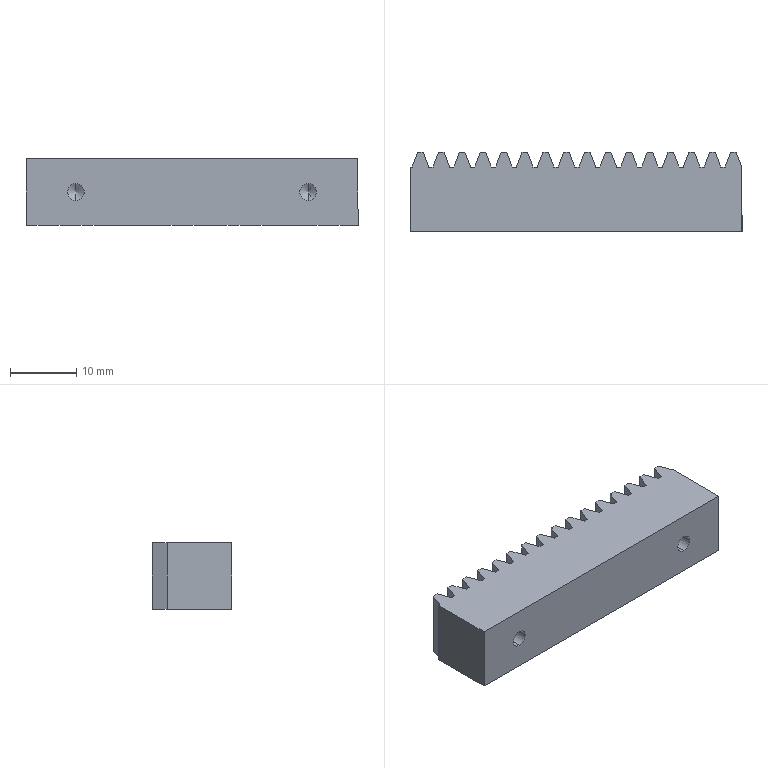Part | SolidWorks | features BaseBody 1, HoleWzd 1, ICE 1 | 1 solid | 78 faces | box 50 x 12 x 10 mm | volume 5397 mm3 | plane 70 | cylinder 4 | cone 4 | commonest cylinder face diameters 2.5 x4